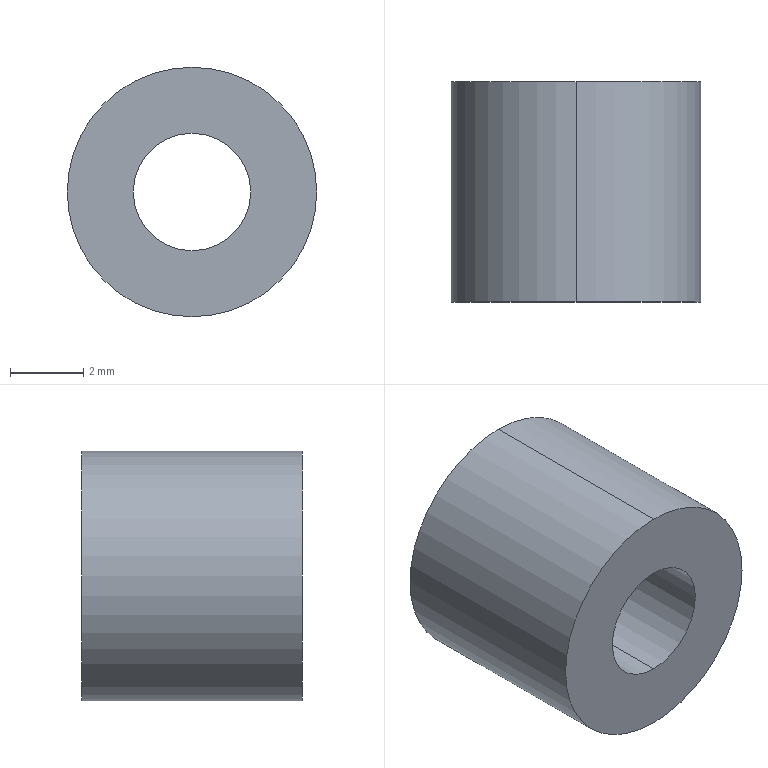Part | SolidWorks | features Extrusion 1 | 1 solid | 6 faces | box 6.8 x 6 x 6.8 mm | volume 169.646 mm3 | cylinder 4 | plane 2 | commonest cylinder face diameters 3.2 x2 6.8 x2
STEP:
#1=CARTESIAN_POINT('',(0.,6.,-1.6));
#2=VERTEX_POINT('',#1);
#3=CARTESIAN_POINT('',(0.,6.,1.6));
#4=VERTEX_POINT('',#3);
#5=CARTESIAN_POINT('',(0.,6.,0.));
#6=DIRECTION('',(0.,1.,0.));
#7=DIRECTION('',(0.,0.,1.));
#8=AXIS2_PLACEMENT_3D('',#5,#6,#7);
#9=CIRCLE('',#8,1.6);
#10=EDGE_CURVE('',#2,#4,#9,.T.);
#11=ORIENTED_EDGE('',*,*,#10,.T.);
#12=CARTESIAN_POINT('',(0.,0.,1.6));
#13=VERTEX_POINT('',#12);
#14=CARTESIAN_POINT('',(0.,6.,1.6));
#15=DIRECTION('',(0.,-1.,0.));
#16=VECTOR('',#15,1000.);
#17=LINE('',#14,#16);
#18=EDGE_CURVE('',#4,#13,#17,.T.);
#19=ORIENTED_EDGE('',*,*,#18,.T.);
#20=CARTESIAN_POINT('',(0.,0.,-1.6));
#21=VERTEX_POINT('',#20);
#22=CARTESIAN_POINT('',(0.,0.,0.));
#23=DIRECTION('',(0.,1.,0.));
#24=DIRECTION('',(0.,0.,1.));
#25=AXIS2_PLACEMENT_3D('',#22,#23,#24);
#26=CIRCLE('',#25,1.6);
#27=EDGE_CURVE('',#21,#13,#26,.T.);
#28=ORIENTED_EDGE('',*,*,#27,.F.);
#29=CARTESIAN_POINT('',(0.,6.,-1.6));
#30=DIRECTION('',(0.,-1.,0.));
#31=VECTOR('',#30,1000.);
#32=LINE('',#29,#31);
#33=EDGE_CURVE('',#2,#21,#32,.T.);
#34=ORIENTED_EDGE('',*,*,#33,.F.);
#35=EDGE_LOOP('',(#11,#19,#28,#34));
#36=FACE_OUTER_BOUND('',#35,.T.);
#37=CARTESIAN_POINT('',(0.,6.,0.));
#38=DIRECTION('',(0.,-1.,0.));
#39=DIRECTION('',(0.,0.,-1.));
#40=AXIS2_PLACEMENT_3D('',#37,#38,#39);
#41=CYLINDRICAL_SURFACE('',#40,1.6);
#42=ADVANCED_FACE('',(#36),#41,.F.);
#43=CARTESIAN_POINT('',(0.,6.,3.4));
#44=VERTEX_POINT('',#43);
#45=CARTESIAN_POINT('',(0.,6.,-3.4));
#46=VERTEX_POINT('',#45);
#47=CARTESIAN_POINT('',(0.,6.,0.));
#48=DIRECTION('',(0.,1.,0.));
#49=DIRECTION('',(0.,0.,1.));
#50=AXIS2_PLACEMENT_3D('',#47,#48,#49);
#51=CIRCLE('',#50,3.4);
#52=EDGE_CURVE('',#44,#46,#51,.T.);
#53=ORIENTED_EDGE('',*,*,#52,.F.);
#54=CARTESIAN_POINT('',(0.,0.,3.4));
#55=VERTEX_POINT('',#54);
#56=CARTESIAN_POINT('',(0.,6.,3.4));
#57=DIRECTION('',(0.,-1.,0.));
#58=VECTOR('',#57,1000.);
#59=LINE('',#56,#58);
#60=EDGE_CURVE('',#44,#55,#59,.T.);
#61=ORIENTED_EDGE('',*,*,#60,.T.);
#62=CARTESIAN_POINT('',(0.,0.,-3.4));
#63=VERTEX_POINT('',#62);
#64=CARTESIAN_POINT('',(0.,0.,0.));
#65=DIRECTION('',(0.,1.,0.));
#66=DIRECTION('',(0.,0.,1.));
#67=AXIS2_PLACEMENT_3D('',#64,#65,#66);
#68=CIRCLE('',#67,3.4);
#69=EDGE_CURVE('',#55,#63,#68,.T.);
#70=ORIENTED_EDGE('',*,*,#69,.T.);
#71=CARTESIAN_POINT('',(0.,6.,-3.4));
#72=DIRECTION('',(0.,-1.,0.));
#73=VECTOR('',#72,1000.);
#74=LINE('',#71,#73);
#75=EDGE_CURVE('',#46,#63,#74,.T.);
#76=ORIENTED_EDGE('',*,*,#75,.F.);
#77=EDGE_LOOP('',(#53,#61,#70,#76));
#78=FACE_OUTER_BOUND('',#77,.T.);
#79=CARTESIAN_POINT('',(0.,6.,0.));
#80=DIRECTION('',(0.,-1.,0.));
#81=DIRECTION('',(0.,0.,-1.));
#82=AXIS2_PLACEMENT_3D('',#79,#80,#81);
#83=CYLINDRICAL_SURFACE('',#82,3.4);
#84=ADVANCED_FACE('',(#78),#83,.T.);
#85=CARTESIAN_POINT('',(0.,6.,0.));
#86=DIRECTION('',(0.,1.,0.));
#87=DIRECTION('',(0.,0.,1.));
#88=AXIS2_PLACEMENT_3D('',#85,#86,#87);
#89=CIRCLE('',#88,3.4);
#90=EDGE_CURVE('',#46,#44,#89,.T.);
#91=ORIENTED_EDGE('',*,*,#90,.T.);
#92=ORIENTED_EDGE('',*,*,#52,.T.);
#93=EDGE_LOOP('',(#91,#92));
#94=FACE_OUTER_BOUND('',#93,.T.);
#95=ORIENTED_EDGE('',*,*,#10,.F.);
#96=CARTESIAN_POINT('',(0.,6.,0.));
#97=DIRECTION('',(0.,1.,0.));
#98=DIRECTION('',(0.,0.,1.));
#99=AXIS2_PLACEMENT_3D('',#96,#97,#98);
#100=CIRCLE('',#99,1.6);
#101=EDGE_CURVE('',#4,#2,#100,.T.);
#102=ORIENTED_EDGE('',*,*,#101,.F.);
#103=EDGE_LOOP('',(#95,#102));
#104=FACE_BOUND('',#103,.T.);
#105=CARTESIAN_POINT('',(0.,6.,0.));
#106=DIRECTION('',(0.,1.,0.));
#107=DIRECTION('',(0.,0.,1.));
#108=AXIS2_PLACEMENT_3D('',#105,#106,#107);
#109=PLANE('',#108);
#110=ADVANCED_FACE('',(#94,#104),#109,.T.);
#111=CARTESIAN_POINT('',(0.,0.,0.));
#112=DIRECTION('',(0.,1.,0.));
#113=DIRECTION('',(0.,0.,1.));
#114=AXIS2_PLACEMENT_3D('',#111,#112,#113);
#115=CIRCLE('',#114,3.4);
#116=EDGE_CURVE('',#63,#55,#115,.T.);
#117=ORIENTED_EDGE('',*,*,#116,.F.);
#118=ORIENTED_EDGE('',*,*,#69,.F.);
#119=EDGE_LOOP('',(#117,#118));
#120=FACE_OUTER_BOUND('',#119,.T.);
#121=ORIENTED_EDGE('',*,*,#27,.T.);
#122=CARTESIAN_POINT('',(0.,0.,0.));
#123=DIRECTION('',(0.,1.,0.));
#124=DIRECTION('',(0.,0.,1.));
#125=AXIS2_PLACEMENT_3D('',#122,#123,#124);
#126=CIRCLE('',#125,1.6);
#127=EDGE_CURVE('',#13,#21,#126,.T.);
#128=ORIENTED_EDGE('',*,*,#127,.T.);
#129=EDGE_LOOP('',(#121,#128));
#130=FACE_BOUND('',#129,.T.);
#131=CARTESIAN_POINT('',(0.,0.,0.));
#132=DIRECTION('',(0.,1.,0.));
#133=DIRECTION('',(0.,0.,1.));
#134=AXIS2_PLACEMENT_3D('',#131,#132,#133);
#135=PLANE('',#134);
#136=ADVANCED_FACE('',(#120,#130),#135,.F.);
#137=ORIENTED_EDGE('',*,*,#60,.F.);
#138=ORIENTED_EDGE('',*,*,#90,.F.);
#139=ORIENTED_EDGE('',*,*,#75,.T.);
#140=ORIENTED_EDGE('',*,*,#116,.T.);
#141=EDGE_LOOP('',(#137,#138,#139,#140));
#142=FACE_OUTER_BOUND('',#141,.T.);
#143=CARTESIAN_POINT('',(0.,6.,0.));
#144=DIRECTION('',(0.,-1.,0.));
#145=DIRECTION('',(0.,0.,-1.));
#146=AXIS2_PLACEMENT_3D('',#143,#144,#145);
#147=CYLINDRICAL_SURFACE('',#146,3.4);
#148=ADVANCED_FACE('',(#142),#147,.T.);
#149=ORIENTED_EDGE('',*,*,#18,.F.);
#150=ORIENTED_EDGE('',*,*,#101,.T.);
#151=ORIENTED_EDGE('',*,*,#33,.T.);
#152=ORIENTED_EDGE('',*,*,#127,.F.);
#153=EDGE_LOOP('',(#149,#150,#151,#152));
#154=FACE_OUTER_BOUND('',#153,.T.);
#155=CARTESIAN_POINT('',(0.,6.,0.));
#156=DIRECTION('',(0.,-1.,0.));
#157=DIRECTION('',(0.,0.,-1.));
#158=AXIS2_PLACEMENT_3D('',#155,#156,#157);
#159=CYLINDRICAL_SURFACE('',#158,1.6);
#160=ADVANCED_FACE('',(#154),#159,.F.);
#161=CLOSED_SHELL('',(#42,#84,#110,#136,#148,#160));
#162=MANIFOLD_SOLID_BREP('',#161);
#163=CARTESIAN_POINT('',(0.,0.,0.));
#164=DIRECTION('',(0.,0.,1.));
#165=DIRECTION('',(1.,0.,0.));
#166=AXIS2_PLACEMENT_3D('',#163,#164,#165);
#167=(LENGTH_UNIT()NAMED_UNIT(*)SI_UNIT(.MILLI.,.METRE.));
#168=UNCERTAINTY_MEASURE_WITH_UNIT(LENGTH_MEASURE(0.00001),#167,'','');
#169=(NAMED_UNIT(*)PLANE_ANGLE_UNIT()SI_UNIT($,.RADIAN.));
#170=(NAMED_UNIT(*)SI_UNIT($,.STERADIAN.)SOLID_ANGLE_UNIT());
#171=(GEOMETRIC_REPRESENTATION_CONTEXT(3)GLOBAL_UNCERTAINTY_ASSIGNED_CONTEXT((#168))GLOBAL_UNIT_ASSIGNED_CONTEXT((#167,#169,#170))REPRESENTATION_CONTEXT('',''));
#172=ADVANCED_BREP_SHAPE_REPRESENTATION('',(#162,#166),#171);